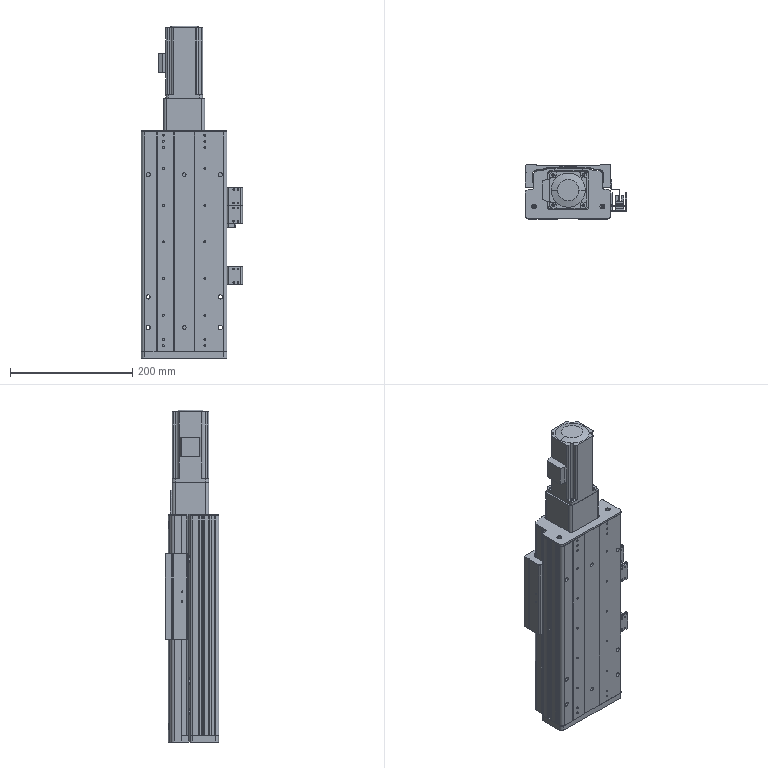Part | SolidWorks | features BaseBody 23 | 23 solids | 1400 faces | box 165.473 x 88 x 543.5 mm | volume 2791596 mm3 | cylinder 707 | plane 615 | cone 78 | commonest cylinder face diameters 8 x106 3.3 x76 4.5 x76 4 x54 6 x50 0.6 x36